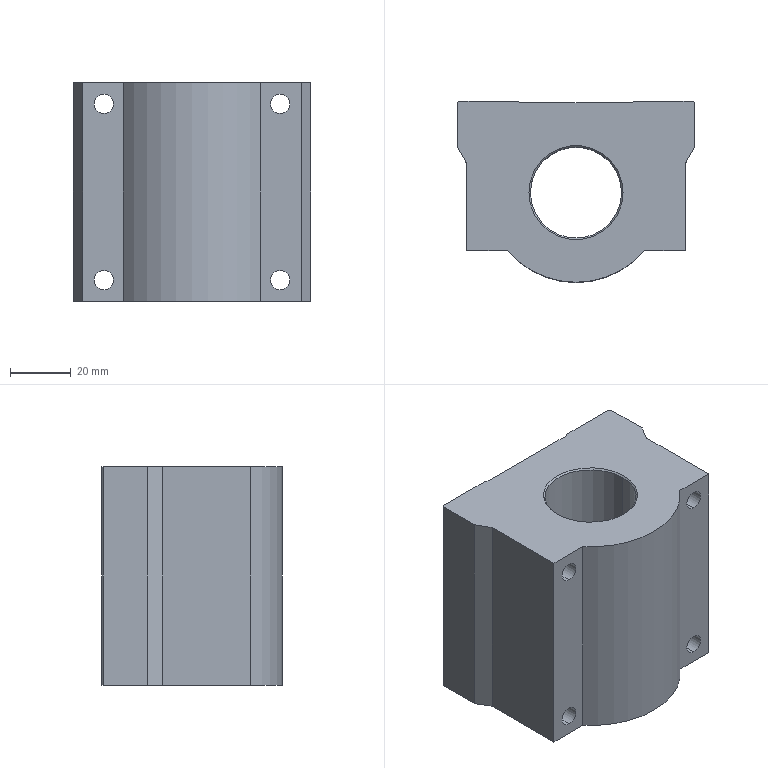Part | SolidWorks | features BaseBody 1 | 1 solid | 400 faces | box 78 x 59.5 x 72 mm | volume 226738 mm3 | plane 242 | spline 124 | cylinder 30 | cone 4 | commonest cylinder face diameters 1.328 x9 2.16 x8 6.4 x8 0.9 x2 30 x2 59 x1